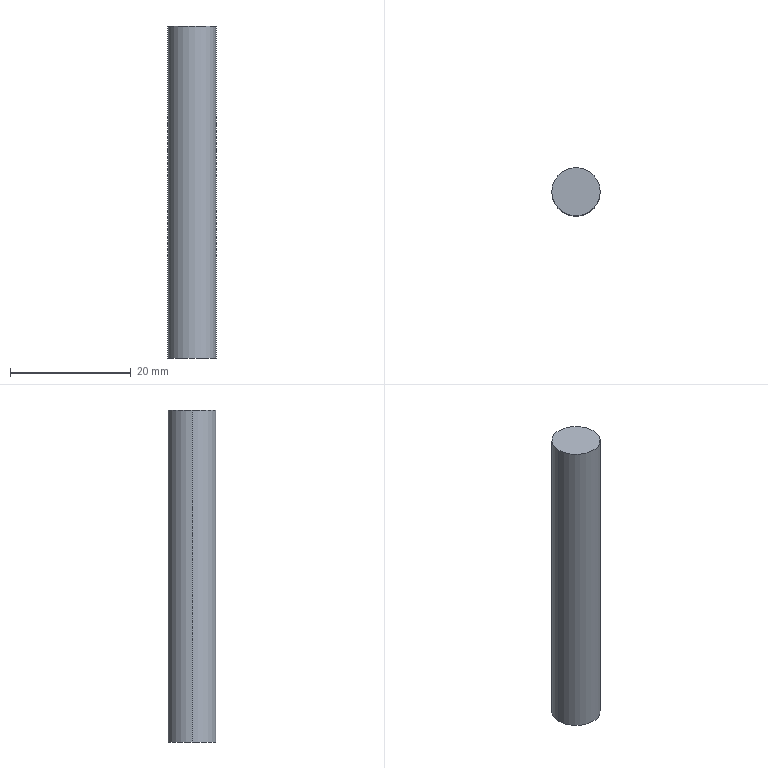Part | SolidWorks | features Extrusion 1 | 1 solid | 4 faces | box 8 x 8 x 55 mm | volume 2765 mm3 | cylinder 2 | plane 2 | commonest cylinder face diameters 8 x2
STEP:
#1=CARTESIAN_POINT('',(4.,0.,27.5));
#2=VERTEX_POINT('',#1);
#3=CARTESIAN_POINT('',(-4.,0.,27.5));
#4=VERTEX_POINT('',#3);
#5=CARTESIAN_POINT('',(0.,0.,27.5));
#6=DIRECTION('',(0.,0.,1.));
#7=DIRECTION('',(1.,0.,0.));
#8=AXIS2_PLACEMENT_3D('',#5,#6,#7);
#9=CIRCLE('',#8,4.);
#10=EDGE_CURVE('',#2,#4,#9,.T.);
#11=ORIENTED_EDGE('',*,*,#10,.F.);
#12=CARTESIAN_POINT('',(4.,0.,-27.5));
#13=VERTEX_POINT('',#12);
#14=CARTESIAN_POINT('',(4.,0.,27.5));
#15=DIRECTION('',(0.,0.,-1.));
#16=VECTOR('',#15,1000.);
#17=LINE('',#14,#16);
#18=EDGE_CURVE('',#2,#13,#17,.T.);
#19=ORIENTED_EDGE('',*,*,#18,.T.);
#20=CARTESIAN_POINT('',(-4.,0.,-27.5));
#21=VERTEX_POINT('',#20);
#22=CARTESIAN_POINT('',(0.,0.,-27.5));
#23=DIRECTION('',(0.,0.,1.));
#24=DIRECTION('',(1.,0.,0.));
#25=AXIS2_PLACEMENT_3D('',#22,#23,#24);
#26=CIRCLE('',#25,4.);
#27=EDGE_CURVE('',#13,#21,#26,.T.);
#28=ORIENTED_EDGE('',*,*,#27,.T.);
#29=CARTESIAN_POINT('',(-4.,0.,27.5));
#30=DIRECTION('',(0.,0.,-1.));
#31=VECTOR('',#30,1000.);
#32=LINE('',#29,#31);
#33=EDGE_CURVE('',#4,#21,#32,.T.);
#34=ORIENTED_EDGE('',*,*,#33,.F.);
#35=EDGE_LOOP('',(#11,#19,#28,#34));
#36=FACE_OUTER_BOUND('',#35,.T.);
#37=CARTESIAN_POINT('',(0.,0.,27.5));
#38=DIRECTION('',(0.,0.,-1.));
#39=DIRECTION('',(-1.,0.,0.));
#40=AXIS2_PLACEMENT_3D('',#37,#38,#39);
#41=CYLINDRICAL_SURFACE('',#40,4.);
#42=ADVANCED_FACE('',(#36),#41,.T.);
#43=ORIENTED_EDGE('',*,*,#18,.F.);
#44=CARTESIAN_POINT('',(0.,0.,27.5));
#45=DIRECTION('',(0.,0.,1.));
#46=DIRECTION('',(1.,0.,0.));
#47=AXIS2_PLACEMENT_3D('',#44,#45,#46);
#48=CIRCLE('',#47,4.);
#49=EDGE_CURVE('',#4,#2,#48,.T.);
#50=ORIENTED_EDGE('',*,*,#49,.F.);
#51=ORIENTED_EDGE('',*,*,#33,.T.);
#52=CARTESIAN_POINT('',(0.,0.,-27.5));
#53=DIRECTION('',(0.,0.,1.));
#54=DIRECTION('',(1.,0.,0.));
#55=AXIS2_PLACEMENT_3D('',#52,#53,#54);
#56=CIRCLE('',#55,4.);
#57=EDGE_CURVE('',#21,#13,#56,.T.);
#58=ORIENTED_EDGE('',*,*,#57,.T.);
#59=EDGE_LOOP('',(#43,#50,#51,#58));
#60=FACE_OUTER_BOUND('',#59,.T.);
#61=CARTESIAN_POINT('',(0.,0.,27.5));
#62=DIRECTION('',(0.,0.,-1.));
#63=DIRECTION('',(-1.,0.,0.));
#64=AXIS2_PLACEMENT_3D('',#61,#62,#63);
#65=CYLINDRICAL_SURFACE('',#64,4.);
#66=ADVANCED_FACE('',(#60),#65,.T.);
#67=ORIENTED_EDGE('',*,*,#49,.T.);
#68=ORIENTED_EDGE('',*,*,#10,.T.);
#69=EDGE_LOOP('',(#67,#68));
#70=FACE_OUTER_BOUND('',#69,.T.);
#71=CARTESIAN_POINT('',(0.,0.,27.5));
#72=DIRECTION('',(0.,0.,1.));
#73=DIRECTION('',(1.,0.,0.));
#74=AXIS2_PLACEMENT_3D('',#71,#72,#73);
#75=PLANE('',#74);
#76=ADVANCED_FACE('',(#70),#75,.T.);
#77=ORIENTED_EDGE('',*,*,#57,.F.);
#78=ORIENTED_EDGE('',*,*,#27,.F.);
#79=EDGE_LOOP('',(#77,#78));
#80=FACE_OUTER_BOUND('',#79,.T.);
#81=CARTESIAN_POINT('',(0.,0.,-27.5));
#82=DIRECTION('',(0.,0.,1.));
#83=DIRECTION('',(1.,0.,0.));
#84=AXIS2_PLACEMENT_3D('',#81,#82,#83);
#85=PLANE('',#84);
#86=ADVANCED_FACE('',(#80),#85,.F.);
#87=CLOSED_SHELL('',(#42,#66,#76,#86));
#88=MANIFOLD_SOLID_BREP('',#87);
#89=CARTESIAN_POINT('',(0.,0.,0.));
#90=DIRECTION('',(0.,0.,1.));
#91=DIRECTION('',(1.,0.,0.));
#92=AXIS2_PLACEMENT_3D('',#89,#90,#91);
#93=(LENGTH_UNIT()NAMED_UNIT(*)SI_UNIT(.MILLI.,.METRE.));
#94=UNCERTAINTY_MEASURE_WITH_UNIT(LENGTH_MEASURE(0.00001),#93,'','');
#95=(NAMED_UNIT(*)PLANE_ANGLE_UNIT()SI_UNIT($,.RADIAN.));
#96=(NAMED_UNIT(*)SI_UNIT($,.STERADIAN.)SOLID_ANGLE_UNIT());
#97=(GEOMETRIC_REPRESENTATION_CONTEXT(3)GLOBAL_UNCERTAINTY_ASSIGNED_CONTEXT((#94))GLOBAL_UNIT_ASSIGNED_CONTEXT((#93,#95,#96))REPRESENTATION_CONTEXT('',''));
#98=ADVANCED_BREP_SHAPE_REPRESENTATION('',(#88,#92),#97);